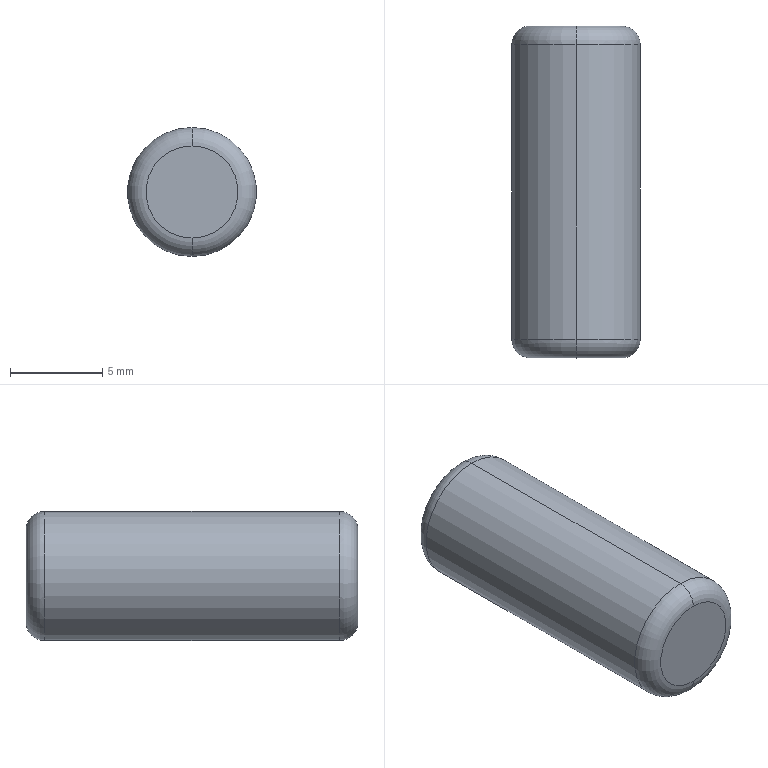Part | SolidWorks | features Extrusion 1, Fillet 1 | 1 solid | 8 faces | box 7 x 18 x 7 mm | volume 683.885 mm3 | torus 4 | cylinder 2 | plane 2 | commonest cylinder face diameters 7 x2
STEP:
#1=CARTESIAN_POINT('',(0.,17.,-3.5));
#2=VERTEX_POINT('',#1);
#3=CARTESIAN_POINT('',(0.,17.,3.5));
#4=VERTEX_POINT('',#3);
#5=CARTESIAN_POINT('',(0.,17.,0.));
#6=DIRECTION('',(0.,-1.,0.));
#7=DIRECTION('',(0.,0.,1.));
#8=AXIS2_PLACEMENT_3D('',#5,#6,#7);
#9=CIRCLE('',#8,3.5);
#10=EDGE_CURVE('',#2,#4,#9,.T.);
#11=ORIENTED_EDGE('',*,*,#10,.F.);
#12=CARTESIAN_POINT('',(0.,18.,-2.5));
#13=VERTEX_POINT('',#12);
#14=CARTESIAN_POINT('',(0.,17.,-2.5));
#15=DIRECTION('',(1.,0.,0.));
#16=DIRECTION('',(0.,0.,-1.));
#17=AXIS2_PLACEMENT_3D('',#14,#15,#16);
#18=CIRCLE('',#17,1.);
#19=EDGE_CURVE('',#2,#13,#18,.T.);
#20=ORIENTED_EDGE('',*,*,#19,.T.);
#21=CARTESIAN_POINT('',(0.,18.,2.5));
#22=VERTEX_POINT('',#21);
#23=CARTESIAN_POINT('',(0.,18.,0.));
#24=DIRECTION('',(0.,1.,0.));
#25=DIRECTION('',(0.,0.,1.));
#26=AXIS2_PLACEMENT_3D('',#23,#24,#25);
#27=CIRCLE('',#26,2.5);
#28=EDGE_CURVE('',#22,#13,#27,.T.);
#29=ORIENTED_EDGE('',*,*,#28,.F.);
#30=CARTESIAN_POINT('',(0.,17.,2.5));
#31=DIRECTION('',(-1.,0.,0.));
#32=DIRECTION('',(0.,0.,1.));
#33=AXIS2_PLACEMENT_3D('',#30,#31,#32);
#34=CIRCLE('',#33,1.);
#35=EDGE_CURVE('',#4,#22,#34,.T.);
#36=ORIENTED_EDGE('',*,*,#35,.F.);
#37=EDGE_LOOP('',(#11,#20,#29,#36));
#38=FACE_OUTER_BOUND('',#37,.T.);
#39=CARTESIAN_POINT('',(0.,17.,0.));
#40=DIRECTION('',(0.,1.,0.));
#41=DIRECTION('',(0.,0.,1.));
#42=AXIS2_PLACEMENT_3D('',#39,#40,#41);
#43=TOROIDAL_SURFACE('',#42,2.5,1.);
#44=ADVANCED_FACE('',(#38),#43,.T.);
#45=CARTESIAN_POINT('',(0.,0.,-2.5));
#46=VERTEX_POINT('',#45);
#47=CARTESIAN_POINT('',(0.,0.,2.5));
#48=VERTEX_POINT('',#47);
#49=CARTESIAN_POINT('',(0.,0.,0.));
#50=DIRECTION('',(0.,-1.,0.));
#51=DIRECTION('',(0.,0.,1.));
#52=AXIS2_PLACEMENT_3D('',#49,#50,#51);
#53=CIRCLE('',#52,2.5);
#54=EDGE_CURVE('',#46,#48,#53,.T.);
#55=ORIENTED_EDGE('',*,*,#54,.F.);
#56=CARTESIAN_POINT('',(0.,1.,-3.5));
#57=VERTEX_POINT('',#56);
#58=CARTESIAN_POINT('',(0.,1.,-2.5));
#59=DIRECTION('',(1.,0.,0.));
#60=DIRECTION('',(0.,0.,-1.));
#61=AXIS2_PLACEMENT_3D('',#58,#59,#60);
#62=CIRCLE('',#61,1.);
#63=EDGE_CURVE('',#46,#57,#62,.T.);
#64=ORIENTED_EDGE('',*,*,#63,.T.);
#65=CARTESIAN_POINT('',(0.,1.,3.5));
#66=VERTEX_POINT('',#65);
#67=CARTESIAN_POINT('',(0.,1.,0.));
#68=DIRECTION('',(0.,1.,0.));
#69=DIRECTION('',(0.,0.,1.));
#70=AXIS2_PLACEMENT_3D('',#67,#68,#69);
#71=CIRCLE('',#70,3.5);
#72=EDGE_CURVE('',#66,#57,#71,.T.);
#73=ORIENTED_EDGE('',*,*,#72,.F.);
#74=CARTESIAN_POINT('',(0.,1.,2.5));
#75=DIRECTION('',(-1.,0.,0.));
#76=DIRECTION('',(0.,0.,1.));
#77=AXIS2_PLACEMENT_3D('',#74,#75,#76);
#78=CIRCLE('',#77,1.);
#79=EDGE_CURVE('',#48,#66,#78,.T.);
#80=ORIENTED_EDGE('',*,*,#79,.F.);
#81=EDGE_LOOP('',(#55,#64,#73,#80));
#82=FACE_OUTER_BOUND('',#81,.T.);
#83=CARTESIAN_POINT('',(0.,1.,0.));
#84=DIRECTION('',(0.,1.,0.));
#85=DIRECTION('',(0.,0.,1.));
#86=AXIS2_PLACEMENT_3D('',#83,#84,#85);
#87=TOROIDAL_SURFACE('',#86,2.5,1.);
#88=ADVANCED_FACE('',(#82),#87,.T.);
#89=ORIENTED_EDGE('',*,*,#10,.T.);
#90=CARTESIAN_POINT('',(0.,18.,3.5));
#91=DIRECTION('',(0.,-1.,0.));
#92=VECTOR('',#91,1000.);
#93=LINE('',#90,#92);
#94=EDGE_CURVE('',#4,#66,#93,.T.);
#95=ORIENTED_EDGE('',*,*,#94,.T.);
#96=ORIENTED_EDGE('',*,*,#72,.T.);
#97=CARTESIAN_POINT('',(0.,18.,-3.5));
#98=DIRECTION('',(0.,-1.,0.));
#99=VECTOR('',#98,1000.);
#100=LINE('',#97,#99);
#101=EDGE_CURVE('',#2,#57,#100,.T.);
#102=ORIENTED_EDGE('',*,*,#101,.F.);
#103=EDGE_LOOP('',(#89,#95,#96,#102));
#104=FACE_OUTER_BOUND('',#103,.T.);
#105=CARTESIAN_POINT('',(0.,18.,0.));
#106=DIRECTION('',(0.,-1.,0.));
#107=DIRECTION('',(0.,0.,-1.));
#108=AXIS2_PLACEMENT_3D('',#105,#106,#107);
#109=CYLINDRICAL_SURFACE('',#108,3.5);
#110=ADVANCED_FACE('',(#104),#109,.T.);
#111=ORIENTED_EDGE('',*,*,#94,.F.);
#112=CARTESIAN_POINT('',(0.,17.,0.));
#113=DIRECTION('',(0.,-1.,0.));
#114=DIRECTION('',(0.,0.,1.));
#115=AXIS2_PLACEMENT_3D('',#112,#113,#114);
#116=CIRCLE('',#115,3.5);
#117=EDGE_CURVE('',#4,#2,#116,.T.);
#118=ORIENTED_EDGE('',*,*,#117,.T.);
#119=ORIENTED_EDGE('',*,*,#101,.T.);
#120=CARTESIAN_POINT('',(0.,1.,0.));
#121=DIRECTION('',(0.,1.,0.));
#122=DIRECTION('',(0.,0.,1.));
#123=AXIS2_PLACEMENT_3D('',#120,#121,#122);
#124=CIRCLE('',#123,3.5);
#125=EDGE_CURVE('',#57,#66,#124,.T.);
#126=ORIENTED_EDGE('',*,*,#125,.T.);
#127=EDGE_LOOP('',(#111,#118,#119,#126));
#128=FACE_OUTER_BOUND('',#127,.T.);
#129=CARTESIAN_POINT('',(0.,18.,0.));
#130=DIRECTION('',(0.,-1.,0.));
#131=DIRECTION('',(0.,0.,-1.));
#132=AXIS2_PLACEMENT_3D('',#129,#130,#131);
#133=CYLINDRICAL_SURFACE('',#132,3.5);
#134=ADVANCED_FACE('',(#128),#133,.T.);
#135=ORIENTED_EDGE('',*,*,#28,.T.);
#136=CARTESIAN_POINT('',(0.,18.,0.));
#137=DIRECTION('',(0.,1.,0.));
#138=DIRECTION('',(0.,0.,1.));
#139=AXIS2_PLACEMENT_3D('',#136,#137,#138);
#140=CIRCLE('',#139,2.5);
#141=EDGE_CURVE('',#13,#22,#140,.T.);
#142=ORIENTED_EDGE('',*,*,#141,.T.);
#143=EDGE_LOOP('',(#135,#142));
#144=FACE_OUTER_BOUND('',#143,.T.);
#145=CARTESIAN_POINT('',(0.,18.,0.));
#146=DIRECTION('',(0.,1.,0.));
#147=DIRECTION('',(0.,0.,1.));
#148=AXIS2_PLACEMENT_3D('',#145,#146,#147);
#149=PLANE('',#148);
#150=ADVANCED_FACE('',(#144),#149,.T.);
#151=CARTESIAN_POINT('',(0.,0.,0.));
#152=DIRECTION('',(0.,-1.,0.));
#153=DIRECTION('',(0.,0.,1.));
#154=AXIS2_PLACEMENT_3D('',#151,#152,#153);
#155=CIRCLE('',#154,2.5);
#156=EDGE_CURVE('',#48,#46,#155,.T.);
#157=ORIENTED_EDGE('',*,*,#156,.T.);
#158=ORIENTED_EDGE('',*,*,#54,.T.);
#159=EDGE_LOOP('',(#157,#158));
#160=FACE_OUTER_BOUND('',#159,.T.);
#161=CARTESIAN_POINT('',(0.,0.,0.));
#162=DIRECTION('',(0.,1.,0.));
#163=DIRECTION('',(0.,0.,1.));
#164=AXIS2_PLACEMENT_3D('',#161,#162,#163);
#165=PLANE('',#164);
#166=ADVANCED_FACE('',(#160),#165,.F.);
#167=ORIENTED_EDGE('',*,*,#63,.F.);
#168=ORIENTED_EDGE('',*,*,#156,.F.);
#169=ORIENTED_EDGE('',*,*,#79,.T.);
#170=ORIENTED_EDGE('',*,*,#125,.F.);
#171=EDGE_LOOP('',(#167,#168,#169,#170));
#172=FACE_OUTER_BOUND('',#171,.T.);
#173=CARTESIAN_POINT('',(0.,1.,0.));
#174=DIRECTION('',(0.,1.,0.));
#175=DIRECTION('',(0.,0.,1.));
#176=AXIS2_PLACEMENT_3D('',#173,#174,#175);
#177=TOROIDAL_SURFACE('',#176,2.5,1.);
#178=ADVANCED_FACE('',(#172),#177,.T.);
#179=ORIENTED_EDGE('',*,*,#19,.F.);
#180=ORIENTED_EDGE('',*,*,#117,.F.);
#181=ORIENTED_EDGE('',*,*,#35,.T.);
#182=ORIENTED_EDGE('',*,*,#141,.F.);
#183=EDGE_LOOP('',(#179,#180,#181,#182));
#184=FACE_OUTER_BOUND('',#183,.T.);
#185=CARTESIAN_POINT('',(0.,17.,0.));
#186=DIRECTION('',(0.,1.,0.));
#187=DIRECTION('',(0.,0.,1.));
#188=AXIS2_PLACEMENT_3D('',#185,#186,#187);
#189=TOROIDAL_SURFACE('',#188,2.5,1.);
#190=ADVANCED_FACE('',(#184),#189,.T.);
#191=CLOSED_SHELL('',(#44,#88,#110,#134,#150,#166,#178,#190));
#192=MANIFOLD_SOLID_BREP('',#191);
#193=CARTESIAN_POINT('',(0.,0.,0.));
#194=DIRECTION('',(0.,0.,1.));
#195=DIRECTION('',(1.,0.,0.));
#196=AXIS2_PLACEMENT_3D('',#193,#194,#195);
#197=(LENGTH_UNIT()NAMED_UNIT(*)SI_UNIT(.MILLI.,.METRE.));
#198=UNCERTAINTY_MEASURE_WITH_UNIT(LENGTH_MEASURE(0.00001),#197,'','');
#199=(NAMED_UNIT(*)PLANE_ANGLE_UNIT()SI_UNIT($,.RADIAN.));
#200=(NAMED_UNIT(*)SI_UNIT($,.STERADIAN.)SOLID_ANGLE_UNIT());
#201=(GEOMETRIC_REPRESENTATION_CONTEXT(3)GLOBAL_UNCERTAINTY_ASSIGNED_CONTEXT((#198))GLOBAL_UNIT_ASSIGNED_CONTEXT((#197,#199,#200))REPRESENTATION_CONTEXT('',''));
#202=ADVANCED_BREP_SHAPE_REPRESENTATION('',(#192,#196),#201);